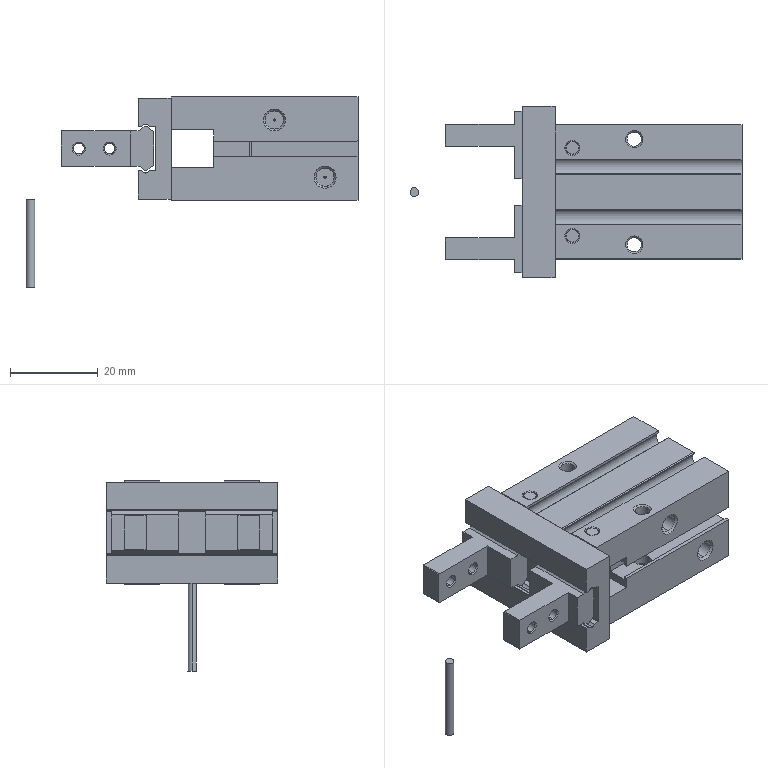Part | SolidWorks | 4 solids | 253 faces | box 75.5 x 39 x 43.25 mm | volume 30245 mm3 | plane 118 | cylinder 73 | cone 62 | commonest cylinder face diameters 3.242 x16 0.4 x10 2.459 x8 1 x6 2 x6 4.02 x6